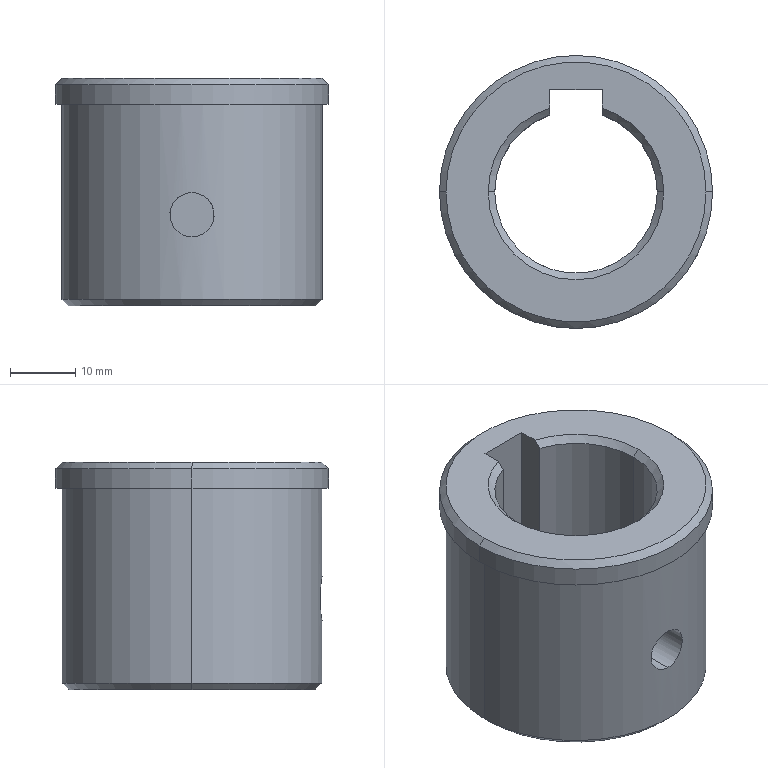Part | SolidWorks | features BaseBody 1 | 1 solid | 25 faces | box 42 x 42 x 35 mm | volume 25861 mm3 | cone 10 | cylinder 9 | plane 6 | commonest cylinder face diameters 25 x3 6.8 x2 40 x2 42 x2
STEP:
#1=CARTESIAN_POINT('',(0.,-12.5,-17.6));
#2=VERTEX_POINT('',#1);
#3=CARTESIAN_POINT('',(0.,-20.,-17.6));
#4=VERTEX_POINT('',#3);
#5=CARTESIAN_POINT('',(0.,-20.,-17.6));
#6=DIRECTION('',(0.,-1.,0.));
#7=VECTOR('',#6,1000.);
#8=LINE('',#5,#7);
#9=EDGE_CURVE('',#2,#4,#8,.T.);
#10=ORIENTED_EDGE('',*,*,#9,.F.);
#11=CARTESIAN_POINT('',(0.,-12.5,-24.4));
#12=VERTEX_POINT('',#11);
#13=CARTESIAN_POINT('',(0.,-12.5,-24.4));
#14=CARTESIAN_POINT('',(0.2239,-12.5,-24.4));
#15=CARTESIAN_POINT('',(0.446,-12.494,-24.378));
#16=CARTESIAN_POINT('',(0.8853,-12.471,-24.29));
#17=CARTESIAN_POINT('',(1.101,-12.453,-24.225));
#18=CARTESIAN_POINT('',(1.716,-12.388,-23.969));
#19=CARTESIAN_POINT('',(2.091,-12.328,-23.718));
#20=CARTESIAN_POINT('',(2.562,-12.236,-23.246));
#21=CARTESIAN_POINT('',(2.701,-12.205,-23.077));
#22=CARTESIAN_POINT('',(2.95,-12.148,-22.706));
#23=CARTESIAN_POINT('',(3.054,-12.122,-22.512));
#24=CARTESIAN_POINT('',(3.226,-12.077,-22.098));
#25=CARTESIAN_POINT('',(3.29,-12.059,-21.885));
#26=CARTESIAN_POINT('',(3.378,-12.035,-21.446));
#27=CARTESIAN_POINT('',(3.4,-12.029,-21.226));
#28=CARTESIAN_POINT('',(3.4,-12.029,-20.889));
#29=CARTESIAN_POINT('',(3.395,-12.03,-20.777));
#30=CARTESIAN_POINT('',(3.373,-12.036,-20.555));
#31=CARTESIAN_POINT('',(3.356,-12.041,-20.443));
#32=CARTESIAN_POINT('',(3.29,-12.059,-20.115));
#33=CARTESIAN_POINT('',(3.225,-12.077,-19.902));
#34=CARTESIAN_POINT('',(2.969,-12.144,-19.285));
#35=CARTESIAN_POINT('',(2.717,-12.205,-18.908));
#36=CARTESIAN_POINT('',(2.247,-12.297,-18.439));
#37=CARTESIAN_POINT('',(2.078,-12.328,-18.299));
#38=CARTESIAN_POINT('',(1.706,-12.384,-18.051));
#39=CARTESIAN_POINT('',(1.51,-12.41,-17.945));
#40=CARTESIAN_POINT('',(1.098,-12.453,-17.774));
#41=CARTESIAN_POINT('',(0.8878,-12.47,-17.71));
#42=CARTESIAN_POINT('',(0.4472,-12.494,-17.622));
#43=CARTESIAN_POINT('',(0.2246,-12.5,-17.6));
#44=CARTESIAN_POINT('',(0.,-12.5,-17.6));
#45=B_SPLINE_CURVE_WITH_KNOTS('',3,(#13,#14,#15,#16,#17,#18,#19,#20,#21,#22,#23,#24,#25,#26,#27,#28,#29,#30,#31,#32,#33,#34,#35,#36,#37,#38,#39,#40,#41,#42,#43,#44),.UNSPECIFIED.,.F.,.F.,(4,2,2,2,2,2,2,2,2,2,2,2,2,2,2,4),(0.,0.0625,0.125,0.25,0.3125,0.375,0.4375,0.5,0.5312,0.5625,0.625,0.75,0.8125,0.875,0.9375,1.),.UNSPECIFIED.);
#46=EDGE_CURVE('',#12,#2,#45,.T.);
#47=ORIENTED_EDGE('',*,*,#46,.F.);
#48=CARTESIAN_POINT('',(0.,-20.,-24.4));
#49=VERTEX_POINT('',#48);
#50=CARTESIAN_POINT('',(0.,-20.,-24.4));
#51=DIRECTION('',(0.,-1.,0.));
#52=VECTOR('',#51,1000.);
#53=LINE('',#50,#52);
#54=EDGE_CURVE('',#12,#49,#53,.T.);
#55=ORIENTED_EDGE('',*,*,#54,.T.);
#56=CARTESIAN_POINT('',(0.,-20.,-24.4));
#57=CARTESIAN_POINT('',(0.2109,-20.,-24.4));
#58=CARTESIAN_POINT('',(0.428,-19.996,-24.38));
#59=CARTESIAN_POINT('',(0.7563,-19.986,-24.317));
#60=CARTESIAN_POINT('',(0.8662,-19.981,-24.29));
#61=CARTESIAN_POINT('',(1.031,-19.973,-24.241));
#62=CARTESIAN_POINT('',(1.113,-19.969,-24.214));
#63=CARTESIAN_POINT('',(1.208,-19.963,-24.178));
#64=CARTESIAN_POINT('',(1.249,-19.961,-24.162));
#65=CARTESIAN_POINT('',(1.276,-19.959,-24.151));
#66=CARTESIAN_POINT('',(1.292,-19.958,-24.145));
#67=CARTESIAN_POINT('',(1.396,-19.951,-24.102));
#68=CARTESIAN_POINT('',(1.492,-19.945,-24.057));
#69=CARTESIAN_POINT('',(1.639,-19.933,-23.979));
#70=CARTESIAN_POINT('',(1.688,-19.929,-23.952));
#71=CARTESIAN_POINT('',(1.763,-19.922,-23.907));
#72=CARTESIAN_POINT('',(1.801,-19.919,-23.884));
#73=CARTESIAN_POINT('',(1.845,-19.915,-23.856));
#74=CARTESIAN_POINT('',(1.867,-19.913,-23.842));
#75=CARTESIAN_POINT('',(1.876,-19.912,-23.835));
#76=CARTESIAN_POINT('',(1.883,-19.911,-23.831));
#77=CARTESIAN_POINT('',(1.887,-19.911,-23.828));
#78=CARTESIAN_POINT('',(1.952,-19.905,-23.785));
#79=CARTESIAN_POINT('',(2.029,-19.897,-23.731));
#80=CARTESIAN_POINT('',(2.203,-19.878,-23.592));
#81=CARTESIAN_POINT('',(2.299,-19.868,-23.509));
#82=CARTESIAN_POINT('',(2.51,-19.842,-23.298));
#83=CARTESIAN_POINT('',(2.595,-19.831,-23.2));
#84=CARTESIAN_POINT('',(2.698,-19.817,-23.07));
#85=CARTESIAN_POINT('',(2.729,-19.813,-23.029));
#86=CARTESIAN_POINT('',(2.769,-19.807,-22.973));
#87=CARTESIAN_POINT('',(2.788,-19.805,-22.946));
#88=CARTESIAN_POINT('',(2.808,-19.802,-22.918));
#89=CARTESIAN_POINT('',(2.817,-19.801,-22.904));
#90=CARTESIAN_POINT('',(2.821,-19.8,-22.898));
#91=CARTESIAN_POINT('',(2.824,-19.8,-22.894));
#92=CARTESIAN_POINT('',(2.824,-19.8,-22.894));
#93=CARTESIAN_POINT('',(2.894,-19.79,-22.789));
#94=CARTESIAN_POINT('',(2.954,-19.781,-22.688));
#95=CARTESIAN_POINT('',(3.032,-19.769,-22.54));
#96=CARTESIAN_POINT('',(3.056,-19.765,-22.492));
#97=CARTESIAN_POINT('',(3.089,-19.76,-22.42));
#98=CARTESIAN_POINT('',(3.106,-19.757,-22.384));
#99=CARTESIAN_POINT('',(3.121,-19.755,-22.349));
#100=CARTESIAN_POINT('',(3.131,-19.753,-22.326));
#101=CARTESIAN_POINT('',(3.135,-19.753,-22.316));
#102=CARTESIAN_POINT('',(3.321,-19.723,-21.868));
#103=CARTESIAN_POINT('',(3.4,-19.709,-21.422));
#104=CARTESIAN_POINT('',(3.4,-19.709,-20.791));
#105=CARTESIAN_POINT('',(3.381,-19.712,-20.574));
#106=CARTESIAN_POINT('',(3.317,-19.723,-20.246));
#107=CARTESIAN_POINT('',(3.29,-19.728,-20.136));
#108=CARTESIAN_POINT('',(3.241,-19.736,-19.972));
#109=CARTESIAN_POINT('',(3.214,-19.74,-19.89));
#110=CARTESIAN_POINT('',(3.179,-19.746,-19.794));
#111=CARTESIAN_POINT('',(3.163,-19.748,-19.753));
#112=CARTESIAN_POINT('',(3.152,-19.75,-19.726));
#113=CARTESIAN_POINT('',(3.146,-19.751,-19.71));
#114=CARTESIAN_POINT('',(3.103,-19.758,-19.606));
#115=CARTESIAN_POINT('',(3.058,-19.765,-19.51));
#116=CARTESIAN_POINT('',(2.98,-19.777,-19.362));
#117=CARTESIAN_POINT('',(2.952,-19.781,-19.312));
#118=CARTESIAN_POINT('',(2.907,-19.788,-19.237));
#119=CARTESIAN_POINT('',(2.884,-19.791,-19.199));
#120=CARTESIAN_POINT('',(2.856,-19.795,-19.155));
#121=CARTESIAN_POINT('',(2.841,-19.797,-19.132));
#122=CARTESIAN_POINT('',(2.835,-19.798,-19.123));
#123=CARTESIAN_POINT('',(2.831,-19.799,-19.117));
#124=CARTESIAN_POINT('',(2.828,-19.799,-19.112));
#125=CARTESIAN_POINT('',(2.786,-19.805,-19.05));
#126=CARTESIAN_POINT('',(2.733,-19.813,-18.974));
#127=CARTESIAN_POINT('',(2.629,-19.827,-18.844));
#128=CARTESIAN_POINT('',(2.591,-19.832,-18.797));
#129=CARTESIAN_POINT('',(2.505,-19.843,-18.7));
#130=CARTESIAN_POINT('',(2.456,-19.849,-18.647));
#131=CARTESIAN_POINT('',(2.301,-19.867,-18.493));
#132=CARTESIAN_POINT('',(2.203,-19.878,-18.408));
#133=CARTESIAN_POINT('',(2.073,-19.892,-18.305));
#134=CARTESIAN_POINT('',(2.032,-19.896,-18.274));
#135=CARTESIAN_POINT('',(1.976,-19.902,-18.233));
#136=CARTESIAN_POINT('',(1.949,-19.905,-18.214));
#137=CARTESIAN_POINT('',(1.919,-19.908,-18.193));
#138=CARTESIAN_POINT('',(1.905,-19.909,-18.184));
#139=CARTESIAN_POINT('',(1.899,-19.91,-18.179));
#140=CARTESIAN_POINT('',(1.895,-19.91,-18.177));
#141=CARTESIAN_POINT('',(1.894,-19.91,-18.176));
#142=CARTESIAN_POINT('',(1.789,-19.92,-18.106));
#143=CARTESIAN_POINT('',(1.688,-19.929,-18.047));
#144=CARTESIAN_POINT('',(1.541,-19.941,-17.969));
#145=CARTESIAN_POINT('',(1.492,-19.944,-17.944));
#146=CARTESIAN_POINT('',(1.42,-19.95,-17.911));
#147=CARTESIAN_POINT('',(1.384,-19.952,-17.894));
#148=CARTESIAN_POINT('',(1.349,-19.954,-17.879));
#149=CARTESIAN_POINT('',(1.325,-19.956,-17.869));
#150=CARTESIAN_POINT('',(1.316,-19.957,-17.865));
#151=CARTESIAN_POINT('',(0.8685,-19.986,-17.679));
#152=CARTESIAN_POINT('',(0.4214,-20.,-17.6));
#153=CARTESIAN_POINT('',(0.,-20.,-17.6));
#154=B_SPLINE_CURVE_WITH_KNOTS('',3,(#56,#57,#58,#59,#60,#61,#62,#63,#64,#65,#66,#67,#68,#69,#70,#71,#72,#73,#74,#75,#76,#77,#78,#79,#80,#81,#82,#83,#84,#85,#86,#87,#88,#89,#90,#91,#92,#93,#94,#95,#96,#97,#98,#99,#100,#101,#102,#103,#104,#105,#106,#107,#108,#109,#110,#111,#112,#113,#114,#115,#116,#117,#118,#119,#120,#121,#122,#123,#124,#125,#126,#127,#128,#129,#130,#131,#132,#133,#134,#135,#136,#137,#138,#139,#140,#141,#142,#143,#144,#145,#146,#147,#148,#149,#150,#151,#152,#153),.UNSPECIFIED.,.F.,.F.,(4,2,2,1,1,2,2,2,2,1,1,1,2,2,2,2,2,2,1,1,1,2,2,2,2,1,2,2,2,2,2,1,1,2,2,2,2,1,1,1,2,2,2,2,2,2,2,1,1,1,2,2,2,2,1,2,2,4),(0.,0.0625,0.09375,0.1094,0.1172,0.1211,0.125,0.1563,0.1719,0.1797,0.1836,0.1855,0.1865,0.1875,0.2188,0.25,0.2813,0.2969,0.3047,0.3086,0.3105,0.3115,0.3125,0.3438,0.3594,0.3672,0.3711,0.375,0.5,0.5625,0.5938,0.6094,0.6172,0.6211,0.625,0.6563,0.6719,0.6797,0.6836,0.6855,0.6865,0.6875,0.7188,0.7344,0.75,0.7813,0.7969,0.8047,0.8086,0.8105,0.8115,0.8125,0.8438,0.8594,0.8672,0.8711,0.875,1.),.UNSPECIFIED.);
#155=EDGE_CURVE('',#49,#4,#154,.T.);
#156=ORIENTED_EDGE('',*,*,#155,.T.);
#157=EDGE_LOOP('',(#10,#47,#55,#156));
#158=FACE_OUTER_BOUND('',#157,.T.);
#159=CARTESIAN_POINT('',(0.,-20.,-21.));
#160=DIRECTION('',(0.,-1.,0.));
#161=DIRECTION('',(0.,0.,-1.));
#162=AXIS2_PLACEMENT_3D('',#159,#160,#161);
#163=CYLINDRICAL_SURFACE('',#162,3.4);
#164=ADVANCED_FACE('',(#158),#163,.F.);
#165=CARTESIAN_POINT('',(-19.,0.,-35.));
#166=VERTEX_POINT('',#165);
#167=CARTESIAN_POINT('',(-20.,0.,-34.));
#168=VERTEX_POINT('',#167);
#169=CARTESIAN_POINT('',(-20.,0.,-34.));
#170=DIRECTION('',(-0.7071,0.,0.7071));
#171=VECTOR('',#170,1000.);
#172=LINE('',#169,#171);
#173=EDGE_CURVE('',#166,#168,#172,.T.);
#174=ORIENTED_EDGE('',*,*,#173,.F.);
#175=CARTESIAN_POINT('',(19.,0.,-35.));
#176=VERTEX_POINT('',#175);
#177=CARTESIAN_POINT('',(0.,0.,-35.));
#178=DIRECTION('',(0.,0.,-1.));
#179=DIRECTION('',(1.,0.,0.));
#180=AXIS2_PLACEMENT_3D('',#177,#178,#179);
#181=CIRCLE('',#180,19.);
#182=EDGE_CURVE('',#176,#166,#181,.T.);
#183=ORIENTED_EDGE('',*,*,#182,.F.);
#184=CARTESIAN_POINT('',(20.,0.,-34.));
#185=VERTEX_POINT('',#184);
#186=CARTESIAN_POINT('',(20.,0.,-34.));
#187=DIRECTION('',(0.7071,0.,0.7071));
#188=VECTOR('',#187,1000.);
#189=LINE('',#186,#188);
#190=EDGE_CURVE('',#176,#185,#189,.T.);
#191=ORIENTED_EDGE('',*,*,#190,.T.);
#192=CARTESIAN_POINT('',(0.,0.,-34.));
#193=DIRECTION('',(0.,0.,1.));
#194=DIRECTION('',(1.,0.,0.));
#195=AXIS2_PLACEMENT_3D('',#192,#193,#194);
#196=CIRCLE('',#195,20.);
#197=EDGE_CURVE('',#168,#185,#196,.T.);
#198=ORIENTED_EDGE('',*,*,#197,.F.);
#199=EDGE_LOOP('',(#174,#183,#191,#198));
#200=FACE_OUTER_BOUND('',#199,.T.);
#201=CARTESIAN_POINT('',(0.,0.,-34.));
#202=DIRECTION('',(0.,0.,1.));
#203=DIRECTION('',(1.,0.,0.));
#204=AXIS2_PLACEMENT_3D('',#201,#202,#203);
#205=CONICAL_SURFACE('',#204,20.,0.7854);
#206=ADVANCED_FACE('',(#200),#205,.T.);
#207=CARTESIAN_POINT('',(12.5,0.,-34.));
#208=VERTEX_POINT('',#207);
#209=CARTESIAN_POINT('',(13.5,0.,-35.));
#210=VERTEX_POINT('',#209);
#211=CARTESIAN_POINT('',(13.5,0.,-35.));
#212=DIRECTION('',(0.7071,0.,-0.7071));
#213=VECTOR('',#212,1000.);
#214=LINE('',#211,#213);
#215=EDGE_CURVE('',#208,#210,#214,.T.);
#216=ORIENTED_EDGE('',*,*,#215,.F.);
#217=CARTESIAN_POINT('',(4.,11.843,-34.));
#218=VERTEX_POINT('',#217);
#219=CARTESIAN_POINT('',(0.,0.,-34.));
#220=DIRECTION('',(0.,0.,-1.));
#221=DIRECTION('',(1.,0.,0.));
#222=AXIS2_PLACEMENT_3D('',#219,#220,#221);
#223=CIRCLE('',#222,12.5);
#224=EDGE_CURVE('',#218,#208,#223,.T.);
#225=ORIENTED_EDGE('',*,*,#224,.F.);
#226=CARTESIAN_POINT('',(4.,12.894,-35.));
#227=VERTEX_POINT('',#226);
#228=CARTESIAN_POINT('',(4.,12.894,-35.));
#229=CARTESIAN_POINT('',(4.,12.544,-34.666));
#230=CARTESIAN_POINT('',(4.,12.194,-34.333));
#231=CARTESIAN_POINT('',(4.,11.843,-34.));
#232=B_SPLINE_CURVE_WITH_KNOTS('',3,(#228,#229,#230,#231),.UNSPECIFIED.,.F.,.F.,(4,4),(0.,0.001451),.UNSPECIFIED.);
#233=EDGE_CURVE('',#227,#218,#232,.T.);
#234=ORIENTED_EDGE('',*,*,#233,.F.);
#235=CARTESIAN_POINT('',(0.,0.,-35.));
#236=DIRECTION('',(0.,0.,1.));
#237=DIRECTION('',(1.,0.,0.));
#238=AXIS2_PLACEMENT_3D('',#235,#236,#237);
#239=CIRCLE('',#238,13.5);
#240=EDGE_CURVE('',#210,#227,#239,.T.);
#241=ORIENTED_EDGE('',*,*,#240,.F.);
#242=EDGE_LOOP('',(#216,#225,#234,#241));
#243=FACE_OUTER_BOUND('',#242,.T.);
#244=CARTESIAN_POINT('',(0.,0.,-35.));
#245=DIRECTION('',(0.,0.,-1.));
#246=DIRECTION('',(-1.,0.,0.));
#247=AXIS2_PLACEMENT_3D('',#244,#245,#246);
#248=CONICAL_SURFACE('',#247,13.5,0.7854);
#249=ADVANCED_FACE('',(#243),#248,.F.);
#250=CARTESIAN_POINT('',(-12.5,0.,-1.));
#251=VERTEX_POINT('',#250);
#252=CARTESIAN_POINT('',(-13.5,0.,0.));
#253=VERTEX_POINT('',#252);
#254=CARTESIAN_POINT('',(-12.5,0.,-1.));
#255=DIRECTION('',(-0.7071,0.,0.7071));
#256=VECTOR('',#255,1000.);
#257=LINE('',#254,#256);
#258=EDGE_CURVE('',#251,#253,#257,.T.);
#259=ORIENTED_EDGE('',*,*,#258,.F.);
#260=CARTESIAN_POINT('',(-4.,11.843,-1.));
#261=VERTEX_POINT('',#260);
#262=CARTESIAN_POINT('',(0.,0.,-1.));
#263=DIRECTION('',(0.,0.,1.));
#264=DIRECTION('',(1.,0.,0.));
#265=AXIS2_PLACEMENT_3D('',#262,#263,#264);
#266=CIRCLE('',#265,12.5);
#267=EDGE_CURVE('',#261,#251,#266,.T.);
#268=ORIENTED_EDGE('',*,*,#267,.F.);
#269=CARTESIAN_POINT('',(-4.,12.894,0.));
#270=VERTEX_POINT('',#269);
#271=CARTESIAN_POINT('',(-4.,12.894,0.));
#272=CARTESIAN_POINT('',(-4.,12.544,-0.334));
#273=CARTESIAN_POINT('',(-4.,12.194,-0.6674));
#274=CARTESIAN_POINT('',(-4.,11.843,-1.));
#275=B_SPLINE_CURVE_WITH_KNOTS('',3,(#271,#272,#273,#274),.UNSPECIFIED.,.F.,.F.,(4,4),(0.,0.001451),.UNSPECIFIED.);
#276=EDGE_CURVE('',#270,#261,#275,.T.);
#277=ORIENTED_EDGE('',*,*,#276,.F.);
#278=CARTESIAN_POINT('',(0.,0.,0.));
#279=DIRECTION('',(0.,0.,-1.));
#280=DIRECTION('',(1.,0.,0.));
#281=AXIS2_PLACEMENT_3D('',#278,#279,#280);
#282=CIRCLE('',#281,13.5);
#283=EDGE_CURVE('',#253,#270,#282,.T.);
#284=ORIENTED_EDGE('',*,*,#283,.F.);
#285=EDGE_LOOP('',(#259,#268,#277,#284));
#286=FACE_OUTER_BOUND('',#285,.T.);
#287=CARTESIAN_POINT('',(0.,0.,-1.));
#288=DIRECTION('',(0.,0.,1.));
#289=DIRECTION('',(1.,0.,0.));
#290=AXIS2_PLACEMENT_3D('',#287,#288,#289);
#291=CONICAL_SURFACE('',#290,12.5,0.7854);
#292=ADVANCED_FACE('',(#286),#291,.F.);
#293=CARTESIAN_POINT('',(20.,0.,0.));
#294=VERTEX_POINT('',#293);
#295=CARTESIAN_POINT('',(21.,0.,-1.));
#296=VERTEX_POINT('',#295);
#297=CARTESIAN_POINT('',(20.,0.,0.));
#298=DIRECTION('',(0.7071,0.,-0.7071));
#299=VECTOR('',#298,1000.);
#300=LINE('',#297,#299);
#301=EDGE_CURVE('',#294,#296,#300,.T.);
#302=ORIENTED_EDGE('',*,*,#301,.F.);
#303=CARTESIAN_POINT('',(-20.,0.,0.));
#304=VERTEX_POINT('',#303);
#305=CARTESIAN_POINT('',(0.,0.,0.));
#306=DIRECTION('',(0.,0.,1.));
#307=DIRECTION('',(1.,0.,0.));
#308=AXIS2_PLACEMENT_3D('',#305,#306,#307);
#309=CIRCLE('',#308,20.);
#310=EDGE_CURVE('',#304,#294,#309,.T.);
#311=ORIENTED_EDGE('',*,*,#310,.F.);
#312=CARTESIAN_POINT('',(-21.,0.,-1.));
#313=VERTEX_POINT('',#312);
#314=CARTESIAN_POINT('',(-20.,0.,0.));
#315=DIRECTION('',(-0.7071,0.,-0.7071));
#316=VECTOR('',#315,1000.);
#317=LINE('',#314,#316);
#318=EDGE_CURVE('',#304,#313,#317,.T.);
#319=ORIENTED_EDGE('',*,*,#318,.T.);
#320=CARTESIAN_POINT('',(0.,0.,-1.));
#321=DIRECTION('',(0.,0.,-1.));
#322=DIRECTION('',(1.,0.,0.));
#323=AXIS2_PLACEMENT_3D('',#320,#321,#322);
#324=CIRCLE('',#323,21.);
#325=EDGE_CURVE('',#296,#313,#324,.T.);
#326=ORIENTED_EDGE('',*,*,#325,.F.);
#327=EDGE_LOOP('',(#302,#311,#319,#326));
#328=FACE_OUTER_BOUND('',#327,.T.);
#329=CARTESIAN_POINT('',(0.,0.,0.));
#330=DIRECTION('',(0.,0.,-1.));
#331=DIRECTION('',(-1.,0.,0.));
#332=AXIS2_PLACEMENT_3D('',#329,#330,#331);
#333=CONICAL_SURFACE('',#332,20.,0.7854);
#334=ADVANCED_FACE('',(#328),#333,.T.);
#335=CARTESIAN_POINT('',(-4.,15.8,-35.));
#336=VERTEX_POINT('',#335);
#337=CARTESIAN_POINT('',(4.,15.8,-35.));
#338=VERTEX_POINT('',#337);
#339=CARTESIAN_POINT('',(4.,15.8,-35.));
#340=DIRECTION('',(1.,0.,0.));
#341=VECTOR('',#340,1000.);
#342=LINE('',#339,#341);
#343=EDGE_CURVE('',#336,#338,#342,.T.);
#344=ORIENTED_EDGE('',*,*,#343,.T.);
#345=CARTESIAN_POINT('',(4.,15.8,0.));
#346=VERTEX_POINT('',#345);
#347=CARTESIAN_POINT('',(4.,15.8,0.));
#348=DIRECTION('',(0.,0.,-1.));
#349=VECTOR('',#348,1000.);
#350=LINE('',#347,#349);
#351=EDGE_CURVE('',#346,#338,#350,.T.);
#352=ORIENTED_EDGE('',*,*,#351,.F.);
#353=CARTESIAN_POINT('',(-4.,15.8,0.));
#354=VERTEX_POINT('',#353);
#355=CARTESIAN_POINT('',(4.,15.8,0.));
#356=DIRECTION('',(1.,0.,0.));
#357=VECTOR('',#356,1000.);
#358=LINE('',#355,#357);
#359=EDGE_CURVE('',#354,#346,#358,.T.);
#360=ORIENTED_EDGE('',*,*,#359,.F.);
#361=CARTESIAN_POINT('',(-4.,15.8,0.));
#362=DIRECTION('',(0.,0.,-1.));
#363=VECTOR('',#362,1000.);
#364=LINE('',#361,#363);
#365=EDGE_CURVE('',#354,#336,#364,.T.);
#366=ORIENTED_EDGE('',*,*,#365,.T.);
#367=EDGE_LOOP('',(#344,#352,#360,#366));
#368=FACE_OUTER_BOUND('',#367,.T.);
#369=CARTESIAN_POINT('',(4.,15.8,0.));
#370=DIRECTION('',(0.,1.,0.));
#371=DIRECTION('',(1.,0.,0.));
#372=AXIS2_PLACEMENT_3D('',#369,#370,#371);
#373=PLANE('',#372);
#374=ADVANCED_FACE('',(#368),#373,.F.);
#375=CARTESIAN_POINT('',(4.,11.843,-1.));
#376=VERTEX_POINT('',#375);
#377=CARTESIAN_POINT('',(4.,11.843,-35.));
#378=DIRECTION('',(0.,0.,-1.));
#379=VECTOR('',#378,1000.);
#380=LINE('',#377,#379);
#381=EDGE_CURVE('',#376,#218,#380,.T.);
#382=ORIENTED_EDGE('',*,*,#381,.F.);
#383=CARTESIAN_POINT('',(4.,12.894,0.));
#384=VERTEX_POINT('',#383);
#385=CARTESIAN_POINT('',(4.,11.843,-1.));
#386=CARTESIAN_POINT('',(4.,12.194,-0.6674));
#387=CARTESIAN_POINT('',(4.,12.544,-0.334));
#388=CARTESIAN_POINT('',(4.,12.894,0.));
#389=B_SPLINE_CURVE_WITH_KNOTS('',3,(#385,#386,#387,#388),.UNSPECIFIED.,.F.,.F.,(4,4),(0.,0.001451),.UNSPECIFIED.);
#390=EDGE_CURVE('',#376,#384,#389,.T.);
#391=ORIENTED_EDGE('',*,*,#390,.T.);
#392=CARTESIAN_POINT('',(4.,15.8,0.));
#393=DIRECTION('',(0.,-1.,0.));
#394=VECTOR('',#393,1000.);
#395=LINE('',#392,#394);
#396=EDGE_CURVE('',#346,#384,#395,.T.);
#397=ORIENTED_EDGE('',*,*,#396,.F.);
#398=ORIENTED_EDGE('',*,*,#351,.T.);
#399=CARTESIAN_POINT('',(4.,15.8,-35.));
#400=DIRECTION('',(0.,-1.,0.));
#401=VECTOR('',#400,1000.);
#402=LINE('',#399,#401);
#403=EDGE_CURVE('',#338,#227,#402,.T.);
#404=ORIENTED_EDGE('',*,*,#403,.T.);
#405=ORIENTED_EDGE('',*,*,#233,.T.);
#406=EDGE_LOOP('',(#382,#391,#397,#398,#404,#405));
#407=FACE_OUTER_BOUND('',#406,.T.);
#408=CARTESIAN_POINT('',(4.,15.8,0.));
#409=DIRECTION('',(1.,0.,0.));
#410=DIRECTION('',(0.,1.,0.));
#411=AXIS2_PLACEMENT_3D('',#408,#409,#410);
#412=PLANE('',#411);
#413=ADVANCED_FACE('',(#407),#412,.F.);
#414=CARTESIAN_POINT('',(-4.,15.8,0.));
#415=DIRECTION('',(0.,1.,0.));
#416=VECTOR('',#415,1000.);
#417=LINE('',#414,#416);
#418=EDGE_CURVE('',#270,#354,#417,.T.);
#419=ORIENTED_EDGE('',*,*,#418,.F.);
#420=ORIENTED_EDGE('',*,*,#276,.T.);
#421=CARTESIAN_POINT('',(-4.,11.843,-34.));
#422=VERTEX_POINT('',#421);
#423=CARTESIAN_POINT('',(-4.,11.843,-35.));
#424=DIRECTION('',(0.,0.,1.));
#425=VECTOR('',#424,1000.);
#426=LINE('',#423,#425);
#427=EDGE_CURVE('',#422,#261,#426,.T.);
#428=ORIENTED_EDGE('',*,*,#427,.F.);
#429=CARTESIAN_POINT('',(-4.,12.894,-35.));
#430=VERTEX_POINT('',#429);
#431=CARTESIAN_POINT('',(-4.,11.843,-34.));
#432=CARTESIAN_POINT('',(-4.,12.194,-34.333));
#433=CARTESIAN_POINT('',(-4.,12.544,-34.666));
#434=CARTESIAN_POINT('',(-4.,12.894,-35.));
#435=B_SPLINE_CURVE_WITH_KNOTS('',3,(#431,#432,#433,#434),.UNSPECIFIED.,.F.,.F.,(4,4),(0.,0.001451),.UNSPECIFIED.);
#436=EDGE_CURVE('',#422,#430,#435,.T.);
#437=ORIENTED_EDGE('',*,*,#436,.T.);
#438=CARTESIAN_POINT('',(-4.,15.8,-35.));
#439=DIRECTION('',(0.,1.,0.));
#440=VECTOR('',#439,1000.);
#441=LINE('',#438,#440);
#442=EDGE_CURVE('',#430,#336,#441,.T.);
#443=ORIENTED_EDGE('',*,*,#442,.T.);
#444=ORIENTED_EDGE('',*,*,#365,.F.);
#445=EDGE_LOOP('',(#419,#420,#428,#437,#443,#444));
#446=FACE_OUTER_BOUND('',#445,.T.);
#447=CARTESIAN_POINT('',(-4.,15.8,0.));
#448=DIRECTION('',(-1.,0.,0.));
#449=DIRECTION('',(0.,0.,1.));
#450=AXIS2_PLACEMENT_3D('',#447,#448,#449);
#451=PLANE('',#450);
#452=ADVANCED_FACE('',(#446),#451,.F.);
#453=CARTESIAN_POINT('',(20.,0.,-4.));
#454=VERTEX_POINT('',#453);
#455=CARTESIAN_POINT('',(-20.,0.,-4.));
#456=VERTEX_POINT('',#455);
#457=CARTESIAN_POINT('',(0.,0.,-4.));
#458=DIRECTION('',(0.,0.,-1.));
#459=DIRECTION('',(1.,0.,0.));
#460=AXIS2_PLACEMENT_3D('',#457,#458,#459);
#461=CIRCLE('',#460,20.);
#462=EDGE_CURVE('',#454,#456,#461,.T.);
#463=ORIENTED_EDGE('',*,*,#462,.F.);
#464=CARTESIAN_POINT('',(0.,0.,-4.));
#465=DIRECTION('',(0.,0.,-1.));
#466=DIRECTION('',(1.,0.,0.));
#467=AXIS2_PLACEMENT_3D('',#464,#465,#466);
#468=CIRCLE('',#467,20.);
#469=EDGE_CURVE('',#456,#454,#468,.T.);
#470=ORIENTED_EDGE('',*,*,#469,.F.);
#471=EDGE_LOOP('',(#463,#470));
#472=FACE_BOUND('',#471,.T.);
#473=CARTESIAN_POINT('',(21.,0.,-4.));
#474=VERTEX_POINT('',#473);
#475=CARTESIAN_POINT('',(-21.,0.,-4.));
#476=VERTEX_POINT('',#475);
#477=CARTESIAN_POINT('',(0.,0.,-4.));
#478=DIRECTION('',(0.,0.,1.));
#479=DIRECTION('',(1.,0.,0.));
#480=AXIS2_PLACEMENT_3D('',#477,#478,#479);
#481=CIRCLE('',#480,21.);
#482=EDGE_CURVE('',#474,#476,#481,.T.);
#483=ORIENTED_EDGE('',*,*,#482,.F.);
#484=CARTESIAN_POINT('',(0.,0.,-4.));
#485=DIRECTION('',(0.,0.,1.));
#486=DIRECTION('',(1.,0.,0.));
#487=AXIS2_PLACEMENT_3D('',#484,#485,#486);
#488=CIRCLE('',#487,21.);
#489=EDGE_CURVE('',#476,#474,#488,.T.);
#490=ORIENTED_EDGE('',*,*,#489,.F.);
#491=EDGE_LOOP('',(#483,#490));
#492=FACE_OUTER_BOUND('',#491,.T.);
#493=CARTESIAN_POINT('',(0.,0.,-4.));
#494=DIRECTION('',(0.,0.,1.));
#495=DIRECTION('',(1.,0.,0.));
#496=AXIS2_PLACEMENT_3D('',#493,#494,#495);
#497=PLANE('',#496);
#498=ADVANCED_FACE('',(#472,#492),#497,.F.);
#499=CARTESIAN_POINT('',(-21.,0.,-4.));
#500=DIRECTION('',(0.,0.,1.));
#501=VECTOR('',#500,1000.);
#502=LINE('',#499,#501);
#503=EDGE_CURVE('',#476,#313,#502,.T.);
#504=ORIENTED_EDGE('',*,*,#503,.F.);
#505=ORIENTED_EDGE('',*,*,#489,.T.);
#506=CARTESIAN_POINT('',(21.,0.,-4.));
#507=DIRECTION('',(0.,0.,1.));
#508=VECTOR('',#507,1000.);
#509=LINE('',#506,#508);
#510=EDGE_CURVE('',#474,#296,#509,.T.);
#511=ORIENTED_EDGE('',*,*,#510,.T.);
#512=ORIENTED_EDGE('',*,*,#325,.T.);
#513=EDGE_LOOP('',(#504,#505,#511,#512));
#514=FACE_OUTER_BOUND('',#513,.T.);
#515=CARTESIAN_POINT('',(0.,0.,-4.));
#516=DIRECTION('',(0.,0.,1.));
#517=DIRECTION('',(1.,0.,0.));
#518=AXIS2_PLACEMENT_3D('',#515,#516,#517);
#519=CYLINDRICAL_SURFACE('',#518,21.);
#520=ADVANCED_FACE('',(#514),#519,.T.);
#521=CARTESIAN_POINT('',(-12.5,0.,-34.));
#522=VERTEX_POINT('',#521);
#523=CARTESIAN_POINT('',(-12.5,0.,-35.));
#524=DIRECTION('',(0.,0.,1.));
#525=VECTOR('',#524,1000.);
#526=LINE('',#523,#525);
#527=EDGE_CURVE('',#522,#251,#526,.T.);
#528=ORIENTED_EDGE('',*,*,#527,.F.);
#529=CARTESIAN_POINT('',(0.,0.,-34.));
#530=DIRECTION('',(0.,0.,-1.));
#531=DIRECTION('',(1.,0.,0.));
#532=AXIS2_PLACEMENT_3D('',#529,#530,#531);
#533=CIRCLE('',#532,12.5);
#534=EDGE_CURVE('',#522,#422,#533,.T.);
#535=ORIENTED_EDGE('',*,*,#534,.T.);
#536=ORIENTED_EDGE('',*,*,#427,.T.);
#537=ORIENTED_EDGE('',*,*,#267,.T.);
#538=EDGE_LOOP('',(#528,#535,#536,#537));
#539=FACE_OUTER_BOUND('',#538,.T.);
#540=CARTESIAN_POINT('',(0.,0.,-35.));
#541=DIRECTION('',(0.,0.,1.));
#542=DIRECTION('',(1.,0.,0.));
#543=AXIS2_PLACEMENT_3D('',#540,#541,#542);
#544=CYLINDRICAL_SURFACE('',#543,12.5);
#545=ADVANCED_FACE('',(#539),#544,.F.);
#546=ORIENTED_EDGE('',*,*,#396,.T.);
#547=CARTESIAN_POINT('',(13.5,0.,0.));
#548=VERTEX_POINT('',#547);
#549=CARTESIAN_POINT('',(0.,0.,0.));
#550=DIRECTION('',(0.,0.,-1.));
#551=DIRECTION('',(1.,0.,0.));
#552=AXIS2_PLACEMENT_3D('',#549,#550,#551);
#553=CIRCLE('',#552,13.5);
#554=EDGE_CURVE('',#384,#548,#553,.T.);
#555=ORIENTED_EDGE('',*,*,#554,.T.);
#556=CARTESIAN_POINT('',(0.,0.,0.));
#557=DIRECTION('',(0.,0.,-1.));
#558=DIRECTION('',(1.,0.,0.));
#559=AXIS2_PLACEMENT_3D('',#556,#557,#558);
#560=CIRCLE('',#559,13.5);
#561=EDGE_CURVE('',#548,#253,#560,.T.);
#562=ORIENTED_EDGE('',*,*,#561,.T.);
#563=ORIENTED_EDGE('',*,*,#283,.T.);
#564=ORIENTED_EDGE('',*,*,#418,.T.);
#565=ORIENTED_EDGE('',*,*,#359,.T.);
#566=EDGE_LOOP('',(#546,#555,#562,#563,#564,#565));
#567=FACE_BOUND('',#566,.T.);
#568=ORIENTED_EDGE('',*,*,#310,.T.);
#569=CARTESIAN_POINT('',(0.,0.,0.));
#570=DIRECTION('',(0.,0.,1.));
#571=DIRECTION('',(1.,0.,0.));
#572=AXIS2_PLACEMENT_3D('',#569,#570,#571);
#573=CIRCLE('',#572,20.);
#574=EDGE_CURVE('',#294,#304,#573,.T.);
#575=ORIENTED_EDGE('',*,*,#574,.T.);
#576=EDGE_LOOP('',(#568,#575));
#577=FACE_OUTER_BOUND('',#576,.T.);
#578=CARTESIAN_POINT('',(0.,0.,0.));
#579=DIRECTION('',(0.,0.,1.));
#580=DIRECTION('',(1.,0.,0.));
#581=AXIS2_PLACEMENT_3D('',#578,#579,#580);
#582=PLANE('',#581);
#583=ADVANCED_FACE('',(#567,#577),#582,.T.);
#584=ORIENTED_EDGE('',*,*,#442,.F.);
#585=CARTESIAN_POINT('',(-13.5,0.,-35.));
#586=VERTEX_POINT('',#585);
#587=CARTESIAN_POINT('',(0.,0.,-35.));
#588=DIRECTION('',(0.,0.,1.));
#589=DIRECTION('',(1.,0.,0.));
#590=AXIS2_PLACEMENT_3D('',#587,#588,#589);
#591=CIRCLE('',#590,13.5);
#592=EDGE_CURVE('',#430,#586,#591,.T.);
#593=ORIENTED_EDGE('',*,*,#592,.T.);
#594=CARTESIAN_POINT('',(0.,0.,-35.));
#595=DIRECTION('',(0.,0.,1.));
#596=DIRECTION('',(1.,0.,0.));
#597=AXIS2_PLACEMENT_3D('',#594,#595,#596);
#598=CIRCLE('',#597,13.5);
#599=EDGE_CURVE('',#586,#210,#598,.T.);
#600=ORIENTED_EDGE('',*,*,#599,.T.);
#601=ORIENTED_EDGE('',*,*,#240,.T.);
#602=ORIENTED_EDGE('',*,*,#403,.F.);
#603=ORIENTED_EDGE('',*,*,#343,.F.);
#604=EDGE_LOOP('',(#584,#593,#600,#601,#602,#603));
#605=FACE_BOUND('',#604,.T.);
#606=ORIENTED_EDGE('',*,*,#182,.T.);
#607=CARTESIAN_POINT('',(0.,0.,-35.));
#608=DIRECTION('',(0.,0.,-1.));
#609=DIRECTION('',(1.,0.,0.));
#610=AXIS2_PLACEMENT_3D('',#607,#608,#609);
#611=CIRCLE('',#610,19.);
#612=EDGE_CURVE('',#166,#176,#611,.T.);
#613=ORIENTED_EDGE('',*,*,#612,.T.);
#614=EDGE_LOOP('',(#606,#613));
#615=FACE_OUTER_BOUND('',#614,.T.);
#616=CARTESIAN_POINT('',(0.,0.,-35.));
#617=DIRECTION('',(0.,0.,1.));
#618=DIRECTION('',(1.,0.,0.));
#619=AXIS2_PLACEMENT_3D('',#616,#617,#618);
#620=PLANE('',#619);
#621=ADVANCED_FACE('',(#605,#615),#620,.F.);
#622=ORIENTED_EDGE('',*,*,#155,.F.);
#623=CARTESIAN_POINT('',(0.,-20.,-17.6));
#624=CARTESIAN_POINT('',(-0.2106,-20.,-17.6));
#625=CARTESIAN_POINT('',(-0.4273,-19.996,-17.62));
#626=CARTESIAN_POINT('',(-0.7551,-19.986,-17.683));
#627=CARTESIAN_POINT('',(-0.8649,-19.981,-17.71));
#628=CARTESIAN_POINT('',(-1.029,-19.974,-17.759));
#629=CARTESIAN_POINT('',(-1.111,-19.969,-17.786));
#630=CARTESIAN_POINT('',(-1.206,-19.964,-17.821));
#631=CARTESIAN_POINT('',(-1.247,-19.961,-17.837));
#632=CARTESIAN_POINT('',(-1.274,-19.959,-17.848));
#633=CARTESIAN_POINT('',(-1.29,-19.958,-17.854));
#634=CARTESIAN_POINT('',(-1.394,-19.952,-17.897));
#635=CARTESIAN_POINT('',(-1.491,-19.945,-17.942));
#636=CARTESIAN_POINT('',(-1.638,-19.933,-18.02));
#637=CARTESIAN_POINT('',(-1.688,-19.929,-18.048));
#638=CARTESIAN_POINT('',(-1.763,-19.922,-18.093));
#639=CARTESIAN_POINT('',(-1.801,-19.919,-18.116));
#640=CARTESIAN_POINT('',(-1.845,-19.915,-18.144));
#641=CARTESIAN_POINT('',(-1.867,-19.913,-18.159));
#642=CARTESIAN_POINT('',(-1.877,-19.912,-18.165));
#643=CARTESIAN_POINT('',(-1.883,-19.911,-18.169));
#644=CARTESIAN_POINT('',(-1.888,-19.911,-18.172));
#645=CARTESIAN_POINT('',(-1.953,-19.905,-18.216));
#646=CARTESIAN_POINT('',(-2.029,-19.897,-18.27));
#647=CARTESIAN_POINT('',(-2.159,-19.883,-18.373));
#648=CARTESIAN_POINT('',(-2.205,-19.878,-18.411));
#649=CARTESIAN_POINT('',(-2.301,-19.867,-18.496));
#650=CARTESIAN_POINT('',(-2.35,-19.862,-18.541));
#651=CARTESIAN_POINT('',(-2.509,-19.842,-18.7));
#652=CARTESIAN_POINT('',(-2.594,-19.831,-18.799));
#653=CARTESIAN_POINT('',(-2.698,-19.817,-18.93));
#654=CARTESIAN_POINT('',(-2.729,-19.813,-18.971));
#655=CARTESIAN_POINT('',(-2.769,-19.807,-19.027));
#656=CARTESIAN_POINT('',(-2.788,-19.805,-19.054));
#657=CARTESIAN_POINT('',(-2.808,-19.802,-19.082));
#658=CARTESIAN_POINT('',(-2.817,-19.801,-19.096));
#659=CARTESIAN_POINT('',(-2.821,-19.8,-19.102));
#660=CARTESIAN_POINT('',(-2.824,-19.8,-19.106));
#661=CARTESIAN_POINT('',(-2.824,-19.8,-19.107));
#662=CARTESIAN_POINT('',(-2.894,-19.79,-19.211));
#663=CARTESIAN_POINT('',(-2.953,-19.781,-19.311));
#664=CARTESIAN_POINT('',(-3.031,-19.769,-19.458));
#665=CARTESIAN_POINT('',(-3.055,-19.765,-19.507));
#666=CARTESIAN_POINT('',(-3.089,-19.76,-19.578));
#667=CARTESIAN_POINT('',(-3.105,-19.758,-19.614));
#668=CARTESIAN_POINT('',(-3.122,-19.755,-19.655));
#669=CARTESIAN_POINT('',(-3.13,-19.754,-19.672));
#670=CARTESIAN_POINT('',(-3.135,-19.753,-19.683));
#671=CARTESIAN_POINT('',(-3.137,-19.752,-19.688));
#672=CARTESIAN_POINT('',(-3.32,-19.723,-20.13));
#673=CARTESIAN_POINT('',(-3.4,-19.709,-20.577));
#674=CARTESIAN_POINT('',(-3.4,-19.709,-21.208));
#675=CARTESIAN_POINT('',(-3.381,-19.712,-21.425));
#676=CARTESIAN_POINT('',(-3.317,-19.723,-21.753));
#677=CARTESIAN_POINT('',(-3.291,-19.728,-21.863));
#678=CARTESIAN_POINT('',(-3.241,-19.736,-22.028));
#679=CARTESIAN_POINT('',(-3.215,-19.74,-22.11));
#680=CARTESIAN_POINT('',(-3.179,-19.746,-22.206));
#681=CARTESIAN_POINT('',(-3.163,-19.748,-22.247));
#682=CARTESIAN_POINT('',(-3.152,-19.75,-22.274));
#683=CARTESIAN_POINT('',(-3.146,-19.751,-22.29));
#684=CARTESIAN_POINT('',(-3.103,-19.758,-22.393));
#685=CARTESIAN_POINT('',(-3.059,-19.765,-22.489));
#686=CARTESIAN_POINT('',(-2.981,-19.777,-22.636));
#687=CARTESIAN_POINT('',(-2.953,-19.781,-22.686));
#688=CARTESIAN_POINT('',(-2.909,-19.787,-22.761));
#689=CARTESIAN_POINT('',(-2.886,-19.791,-22.798));
#690=CARTESIAN_POINT('',(-2.858,-19.795,-22.842));
#691=CARTESIAN_POINT('',(-2.843,-19.797,-22.865));
#692=CARTESIAN_POINT('',(-2.837,-19.798,-22.874));
#693=CARTESIAN_POINT('',(-2.833,-19.798,-22.88));
#694=CARTESIAN_POINT('',(-2.83,-19.799,-22.885));
#695=CARTESIAN_POINT('',(-2.788,-19.805,-22.948));
#696=CARTESIAN_POINT('',(-2.735,-19.812,-23.023));
#697=CARTESIAN_POINT('',(-2.631,-19.826,-23.154));
#698=CARTESIAN_POINT('',(-2.592,-19.831,-23.201));
#699=CARTESIAN_POINT('',(-2.506,-19.842,-23.299));
#700=CARTESIAN_POINT('',(-2.457,-19.849,-23.351));
#701=CARTESIAN_POINT('',(-2.302,-19.867,-23.506));
#702=CARTESIAN_POINT('',(-2.205,-19.878,-23.59));
#703=CARTESIAN_POINT('',(-2.075,-19.892,-23.694));
#704=CARTESIAN_POINT('',(-2.034,-19.896,-23.725));
#705=CARTESIAN_POINT('',(-1.977,-19.902,-23.766));
#706=CARTESIAN_POINT('',(-1.95,-19.905,-23.785));
#707=CARTESIAN_POINT('',(-1.921,-19.908,-23.806));
#708=CARTESIAN_POINT('',(-1.906,-19.909,-23.815));
#709=CARTESIAN_POINT('',(-1.9,-19.909,-23.819));
#710=CARTESIAN_POINT('',(-1.897,-19.91,-23.822));
#711=CARTESIAN_POINT('',(-1.896,-19.91,-23.822));
#712=CARTESIAN_POINT('',(-1.791,-19.92,-23.892));
#713=CARTESIAN_POINT('',(-1.691,-19.929,-23.952));
#714=CARTESIAN_POINT('',(-1.544,-19.94,-24.03));
#715=CARTESIAN_POINT('',(-1.495,-19.944,-24.054));
#716=CARTESIAN_POINT('',(-1.423,-19.949,-24.088));
#717=CARTESIAN_POINT('',(-1.388,-19.952,-24.104));
#718=CARTESIAN_POINT('',(-1.352,-19.954,-24.119));
#719=CARTESIAN_POINT('',(-1.329,-19.956,-24.129));
#720=CARTESIAN_POINT('',(-1.319,-19.956,-24.134));
#721=CARTESIAN_POINT('',(-0.8711,-19.986,-24.32));
#722=CARTESIAN_POINT('',(-0.4226,-20.,-24.4));
#723=CARTESIAN_POINT('',(0.,-20.,-24.4));
#724=B_SPLINE_CURVE_WITH_KNOTS('',3,(#623,#624,#625,#626,#627,#628,#629,#630,#631,#632,#633,#634,#635,#636,#637,#638,#639,#640,#641,#642,#643,#644,#645,#646,#647,#648,#649,#650,#651,#652,#653,#654,#655,#656,#657,#658,#659,#660,#661,#662,#663,#664,#665,#666,#667,#668,#669,#670,#671,#672,#673,#674,#675,#676,#677,#678,#679,#680,#681,#682,#683,#684,#685,#686,#687,#688,#689,#690,#691,#692,#693,#694,#695,#696,#697,#698,#699,#700,#701,#702,#703,#704,#705,#706,#707,#708,#709,#710,#711,#712,#713,#714,#715,#716,#717,#718,#719,#720,#721,#722,#723),.UNSPECIFIED.,.F.,.F.,(4,2,2,1,1,2,2,2,2,1,1,1,2,2,2,2,2,2,2,1,1,1,2,2,2,2,1,1,2,2,2,2,2,1,1,2,2,2,2,1,1,1,2,2,2,2,2,2,2,1,1,1,2,2,2,2,1,2,2,4),(0.,0.0625,0.09375,0.1094,0.1172,0.1211,0.125,0.1563,0.1719,0.1797,0.1836,0.1855,0.1865,0.1875,0.2188,0.2344,0.25,0.2813,0.2969,0.3047,0.3086,0.3105,0.3115,0.3125,0.3438,0.3594,0.3672,0.3711,0.373,0.375,0.5,0.5625,0.5937,0.6094,0.6172,0.6211,0.625,0.6562,0.6719,0.6797,0.6836,0.6855,0.6865,0.6875,0.7187,0.7344,0.75,0.7812,0.7969,0.8047,0.8086,0.8105,0.8115,0.8125,0.8437,0.8594,0.8672,0.8711,0.875,1.),.UNSPECIFIED.);
#725=EDGE_CURVE('',#4,#49,#724,.T.);
#726=ORIENTED_EDGE('',*,*,#725,.F.);
#727=EDGE_LOOP('',(#622,#726));
#728=FACE_BOUND('',#727,.T.);
#729=CARTESIAN_POINT('',(-20.,0.,-35.));
#730=DIRECTION('',(0.,0.,1.));
#731=VECTOR('',#730,1000.);
#732=LINE('',#729,#731);
#733=EDGE_CURVE('',#168,#456,#732,.T.);
#734=ORIENTED_EDGE('',*,*,#733,.F.);
#735=ORIENTED_EDGE('',*,*,#197,.T.);
#736=CARTESIAN_POINT('',(20.,0.,-35.));
#737=DIRECTION('',(0.,0.,1.));
#738=VECTOR('',#737,1000.);
#739=LINE('',#736,#738);
#740=EDGE_CURVE('',#185,#454,#739,.T.);
#741=ORIENTED_EDGE('',*,*,#740,.T.);
#742=ORIENTED_EDGE('',*,*,#462,.T.);
#743=EDGE_LOOP('',(#734,#735,#741,#742));
#744=FACE_OUTER_BOUND('',#743,.T.);
#745=CARTESIAN_POINT('',(0.,0.,-35.));
#746=DIRECTION('',(0.,0.,1.));
#747=DIRECTION('',(1.,0.,0.));
#748=AXIS2_PLACEMENT_3D('',#745,#746,#747);
#749=CYLINDRICAL_SURFACE('',#748,20.);
#750=ADVANCED_FACE('',(#728,#744),#749,.T.);
#751=CARTESIAN_POINT('',(0.,0.,-34.));
#752=DIRECTION('',(0.,0.,1.));
#753=DIRECTION('',(1.,0.,0.));
#754=AXIS2_PLACEMENT_3D('',#751,#752,#753);
#755=CIRCLE('',#754,20.);
#756=EDGE_CURVE('',#185,#168,#755,.T.);
#757=ORIENTED_EDGE('',*,*,#756,.T.);
#758=ORIENTED_EDGE('',*,*,#733,.T.);
#759=ORIENTED_EDGE('',*,*,#469,.T.);
#760=ORIENTED_EDGE('',*,*,#740,.F.);
#761=EDGE_LOOP('',(#757,#758,#759,#760));
#762=FACE_OUTER_BOUND('',#761,.T.);
#763=CARTESIAN_POINT('',(0.,0.,-35.));
#764=DIRECTION('',(0.,0.,1.));
#765=DIRECTION('',(1.,0.,0.));
#766=AXIS2_PLACEMENT_3D('',#763,#764,#765);
#767=CYLINDRICAL_SURFACE('',#766,20.);
#768=ADVANCED_FACE('',(#762),#767,.T.);
#769=ORIENTED_EDGE('',*,*,#224,.T.);
#770=CARTESIAN_POINT('',(12.5,0.,-1.));
#771=VERTEX_POINT('',#770);
#772=CARTESIAN_POINT('',(12.5,0.,-35.));
#773=DIRECTION('',(0.,0.,1.));
#774=VECTOR('',#773,1000.);
#775=LINE('',#772,#774);
#776=EDGE_CURVE('',#208,#771,#775,.T.);
#777=ORIENTED_EDGE('',*,*,#776,.T.);
#778=CARTESIAN_POINT('',(0.,0.,-1.));
#779=DIRECTION('',(0.,0.,1.));
#780=DIRECTION('',(1.,0.,0.));
#781=AXIS2_PLACEMENT_3D('',#778,#779,#780);
#782=CIRCLE('',#781,12.5);
#783=EDGE_CURVE('',#771,#376,#782,.T.);
#784=ORIENTED_EDGE('',*,*,#783,.T.);
#785=ORIENTED_EDGE('',*,*,#381,.T.);
#786=EDGE_LOOP('',(#769,#777,#784,#785));
#787=FACE_OUTER_BOUND('',#786,.T.);
#788=CARTESIAN_POINT('',(0.,0.,-35.));
#789=DIRECTION('',(0.,0.,1.));
#790=DIRECTION('',(1.,0.,0.));
#791=AXIS2_PLACEMENT_3D('',#788,#789,#790);
#792=CYLINDRICAL_SURFACE('',#791,12.5);
#793=ADVANCED_FACE('',(#787),#792,.F.);
#794=ORIENTED_EDGE('',*,*,#46,.T.);
#795=CARTESIAN_POINT('',(0.,-12.5,-17.6));
#796=CARTESIAN_POINT('',(-0.4479,-12.5,-17.6));
#797=CARTESIAN_POINT('',(-0.8914,-12.475,-17.689));
#798=CARTESIAN_POINT('',(-1.51,-12.41,-17.946));
#799=CARTESIAN_POINT('',(-1.708,-12.384,-18.052));
#800=CARTESIAN_POINT('',(-2.076,-12.328,-18.298));
#801=CARTESIAN_POINT('',(-2.246,-12.298,-18.437));
#802=CARTESIAN_POINT('',(-2.561,-12.236,-18.753));
#803=CARTESIAN_POINT('',(-2.702,-12.205,-18.924));
#804=CARTESIAN_POINT('',(-2.95,-12.148,-19.294));
#805=CARTESIAN_POINT('',(-3.053,-12.122,-19.488));
#806=CARTESIAN_POINT('',(-3.225,-12.077,-19.901));
#807=CARTESIAN_POINT('',(-3.29,-12.059,-20.112));
#808=CARTESIAN_POINT('',(-3.378,-12.035,-20.552));
#809=CARTESIAN_POINT('',(-3.4,-12.029,-20.776));
#810=CARTESIAN_POINT('',(-3.4,-12.029,-21.222));
#811=CARTESIAN_POINT('',(-3.378,-12.035,-21.444));
#812=CARTESIAN_POINT('',(-3.313,-12.053,-21.773));
#813=CARTESIAN_POINT('',(-3.286,-12.06,-21.881));
#814=CARTESIAN_POINT('',(-3.221,-12.078,-22.095));
#815=CARTESIAN_POINT('',(-3.183,-12.088,-22.201));
#816=CARTESIAN_POINT('',(-2.97,-12.143,-22.714));
#817=CARTESIAN_POINT('',(-2.72,-12.205,-23.088));
#818=CARTESIAN_POINT('',(-2.248,-12.297,-23.56));
#819=CARTESIAN_POINT('',(-2.076,-12.328,-23.701));
#820=CARTESIAN_POINT('',(-1.8,-12.37,-23.887));
#821=CARTESIAN_POINT('',(-1.705,-12.384,-23.944));
#822=CARTESIAN_POINT('',(-1.51,-12.409,-24.048));
#823=CARTESIAN_POINT('',(-1.411,-12.421,-24.095));
#824=CARTESIAN_POINT('',(-0.8933,-12.475,-24.311));
#825=CARTESIAN_POINT('',(-0.4488,-12.5,-24.4));
#826=CARTESIAN_POINT('',(0.,-12.5,-24.4));
#827=B_SPLINE_CURVE_WITH_KNOTS('',3,(#795,#796,#797,#798,#799,#800,#801,#802,#803,#804,#805,#806,#807,#808,#809,#810,#811,#812,#813,#814,#815,#816,#817,#818,#819,#820,#821,#822,#823,#824,#825,#826),.UNSPECIFIED.,.F.,.F.,(4,2,2,2,2,2,2,2,2,2,2,2,2,2,2,4),(0.,0.125,0.1875,0.25,0.3125,0.375,0.4375,0.5,0.5625,0.5937,0.625,0.75,0.8125,0.8438,0.875,1.),.UNSPECIFIED.);
#828=EDGE_CURVE('',#2,#12,#827,.T.);
#829=ORIENTED_EDGE('',*,*,#828,.T.);
#830=EDGE_LOOP('',(#794,#829));
#831=FACE_BOUND('',#830,.T.);
#832=CARTESIAN_POINT('',(0.,0.,-34.));
#833=DIRECTION('',(0.,0.,-1.));
#834=DIRECTION('',(1.,0.,0.));
#835=AXIS2_PLACEMENT_3D('',#832,#833,#834);
#836=CIRCLE('',#835,12.5);
#837=EDGE_CURVE('',#208,#522,#836,.T.);
#838=ORIENTED_EDGE('',*,*,#837,.T.);
#839=ORIENTED_EDGE('',*,*,#527,.T.);
#840=CARTESIAN_POINT('',(0.,0.,-1.));
#841=DIRECTION('',(0.,0.,1.));
#842=DIRECTION('',(1.,0.,0.));
#843=AXIS2_PLACEMENT_3D('',#840,#841,#842);
#844=CIRCLE('',#843,12.5);
#845=EDGE_CURVE('',#251,#771,#844,.T.);
#846=ORIENTED_EDGE('',*,*,#845,.T.);
#847=ORIENTED_EDGE('',*,*,#776,.F.);
#848=EDGE_LOOP('',(#838,#839,#846,#847));
#849=FACE_OUTER_BOUND('',#848,.T.);
#850=CARTESIAN_POINT('',(0.,0.,-35.));
#851=DIRECTION('',(0.,0.,1.));
#852=DIRECTION('',(1.,0.,0.));
#853=AXIS2_PLACEMENT_3D('',#850,#851,#852);
#854=CYLINDRICAL_SURFACE('',#853,12.5);
#855=ADVANCED_FACE('',(#831,#849),#854,.F.);
#856=ORIENTED_EDGE('',*,*,#482,.T.);
#857=ORIENTED_EDGE('',*,*,#503,.T.);
#858=CARTESIAN_POINT('',(0.,0.,-1.));
#859=DIRECTION('',(0.,0.,-1.));
#860=DIRECTION('',(1.,0.,0.));
#861=AXIS2_PLACEMENT_3D('',#858,#859,#860);
#862=CIRCLE('',#861,21.);
#863=EDGE_CURVE('',#313,#296,#862,.T.);
#864=ORIENTED_EDGE('',*,*,#863,.T.);
#865=ORIENTED_EDGE('',*,*,#510,.F.);
#866=EDGE_LOOP('',(#856,#857,#864,#865));
#867=FACE_OUTER_BOUND('',#866,.T.);
#868=CARTESIAN_POINT('',(0.,0.,-4.));
#869=DIRECTION('',(0.,0.,1.));
#870=DIRECTION('',(1.,0.,0.));
#871=AXIS2_PLACEMENT_3D('',#868,#869,#870);
#872=CYLINDRICAL_SURFACE('',#871,21.);
#873=ADVANCED_FACE('',(#867),#872,.T.);
#874=ORIENTED_EDGE('',*,*,#574,.F.);
#875=ORIENTED_EDGE('',*,*,#301,.T.);
#876=ORIENTED_EDGE('',*,*,#863,.F.);
#877=ORIENTED_EDGE('',*,*,#318,.F.);
#878=EDGE_LOOP('',(#874,#875,#876,#877));
#879=FACE_OUTER_BOUND('',#878,.T.);
#880=CARTESIAN_POINT('',(0.,0.,0.));
#881=DIRECTION('',(0.,0.,-1.));
#882=DIRECTION('',(-1.,0.,0.));
#883=AXIS2_PLACEMENT_3D('',#880,#881,#882);
#884=CONICAL_SURFACE('',#883,20.,0.7854);
#885=ADVANCED_FACE('',(#879),#884,.T.);
#886=ORIENTED_EDGE('',*,*,#783,.F.);
#887=CARTESIAN_POINT('',(12.5,0.,-1.));
#888=DIRECTION('',(0.7071,0.,0.7071));
#889=VECTOR('',#888,1000.);
#890=LINE('',#887,#889);
#891=EDGE_CURVE('',#771,#548,#890,.T.);
#892=ORIENTED_EDGE('',*,*,#891,.T.);
#893=ORIENTED_EDGE('',*,*,#554,.F.);
#894=ORIENTED_EDGE('',*,*,#390,.F.);
#895=EDGE_LOOP('',(#886,#892,#893,#894));
#896=FACE_OUTER_BOUND('',#895,.T.);
#897=CARTESIAN_POINT('',(0.,0.,-1.));
#898=DIRECTION('',(0.,0.,1.));
#899=DIRECTION('',(1.,0.,0.));
#900=AXIS2_PLACEMENT_3D('',#897,#898,#899);
#901=CONICAL_SURFACE('',#900,12.5,0.7854);
#902=ADVANCED_FACE('',(#896),#901,.F.);
#903=ORIENTED_EDGE('',*,*,#845,.F.);
#904=ORIENTED_EDGE('',*,*,#258,.T.);
#905=ORIENTED_EDGE('',*,*,#561,.F.);
#906=ORIENTED_EDGE('',*,*,#891,.F.);
#907=EDGE_LOOP('',(#903,#904,#905,#906));
#908=FACE_OUTER_BOUND('',#907,.T.);
#909=CARTESIAN_POINT('',(0.,0.,-1.));
#910=DIRECTION('',(0.,0.,1.));
#911=DIRECTION('',(1.,0.,0.));
#912=AXIS2_PLACEMENT_3D('',#909,#910,#911);
#913=CONICAL_SURFACE('',#912,12.5,0.7854);
#914=ADVANCED_FACE('',(#908),#913,.F.);
#915=ORIENTED_EDGE('',*,*,#534,.F.);
#916=CARTESIAN_POINT('',(-13.5,0.,-35.));
#917=DIRECTION('',(-0.7071,0.,-0.7071));
#918=VECTOR('',#917,1000.);
#919=LINE('',#916,#918);
#920=EDGE_CURVE('',#522,#586,#919,.T.);
#921=ORIENTED_EDGE('',*,*,#920,.T.);
#922=ORIENTED_EDGE('',*,*,#592,.F.);
#923=ORIENTED_EDGE('',*,*,#436,.F.);
#924=EDGE_LOOP('',(#915,#921,#922,#923));
#925=FACE_OUTER_BOUND('',#924,.T.);
#926=CARTESIAN_POINT('',(0.,0.,-35.));
#927=DIRECTION('',(0.,0.,-1.));
#928=DIRECTION('',(-1.,0.,0.));
#929=AXIS2_PLACEMENT_3D('',#926,#927,#928);
#930=CONICAL_SURFACE('',#929,13.5,0.7854);
#931=ADVANCED_FACE('',(#925),#930,.F.);
#932=ORIENTED_EDGE('',*,*,#837,.F.);
#933=ORIENTED_EDGE('',*,*,#215,.T.);
#934=ORIENTED_EDGE('',*,*,#599,.F.);
#935=ORIENTED_EDGE('',*,*,#920,.F.);
#936=EDGE_LOOP('',(#932,#933,#934,#935));
#937=FACE_OUTER_BOUND('',#936,.T.);
#938=CARTESIAN_POINT('',(0.,0.,-35.));
#939=DIRECTION('',(0.,0.,-1.));
#940=DIRECTION('',(-1.,0.,0.));
#941=AXIS2_PLACEMENT_3D('',#938,#939,#940);
#942=CONICAL_SURFACE('',#941,13.5,0.7854);
#943=ADVANCED_FACE('',(#937),#942,.F.);
#944=ORIENTED_EDGE('',*,*,#612,.F.);
#945=ORIENTED_EDGE('',*,*,#173,.T.);
#946=ORIENTED_EDGE('',*,*,#756,.F.);
#947=ORIENTED_EDGE('',*,*,#190,.F.);
#948=EDGE_LOOP('',(#944,#945,#946,#947));
#949=FACE_OUTER_BOUND('',#948,.T.);
#950=CARTESIAN_POINT('',(0.,0.,-34.));
#951=DIRECTION('',(0.,0.,1.));
#952=DIRECTION('',(1.,0.,0.));
#953=AXIS2_PLACEMENT_3D('',#950,#951,#952);
#954=CONICAL_SURFACE('',#953,20.,0.7854);
#955=ADVANCED_FACE('',(#949),#954,.T.);
#956=ORIENTED_EDGE('',*,*,#828,.F.);
#957=ORIENTED_EDGE('',*,*,#9,.T.);
#958=ORIENTED_EDGE('',*,*,#725,.T.);
#959=ORIENTED_EDGE('',*,*,#54,.F.);
#960=EDGE_LOOP('',(#956,#957,#958,#959));
#961=FACE_OUTER_BOUND('',#960,.T.);
#962=CARTESIAN_POINT('',(0.,-20.,-21.));
#963=DIRECTION('',(0.,-1.,0.));
#964=DIRECTION('',(0.,0.,-1.));
#965=AXIS2_PLACEMENT_3D('',#962,#963,#964);
#966=CYLINDRICAL_SURFACE('',#965,3.4);
#967=ADVANCED_FACE('',(#961),#966,.F.);
#968=CLOSED_SHELL('',(#164,#206,#249,#292,#334,#374,#413,#452,#498,#520,#545,#583,#621,#750,#768,#793,#855,#873,#885,#902,#914,#931,#943,#955,#967));
#969=MANIFOLD_SOLID_BREP('',#968);
#970=CARTESIAN_POINT('',(0.,0.,0.));
#971=DIRECTION('',(0.,0.,1.));
#972=DIRECTION('',(1.,0.,0.));
#973=AXIS2_PLACEMENT_3D('',#970,#971,#972);
#974=(LENGTH_UNIT()NAMED_UNIT(*)SI_UNIT(.MILLI.,.METRE.));
#975=UNCERTAINTY_MEASURE_WITH_UNIT(LENGTH_MEASURE(0.00001),#974,'','');
#976=(NAMED_UNIT(*)PLANE_ANGLE_UNIT()SI_UNIT($,.RADIAN.));
#977=(NAMED_UNIT(*)SI_UNIT($,.STERADIAN.)SOLID_ANGLE_UNIT());
#978=(GEOMETRIC_REPRESENTATION_CONTEXT(3)GLOBAL_UNCERTAINTY_ASSIGNED_CONTEXT((#975))GLOBAL_UNIT_ASSIGNED_CONTEXT((#974,#976,#977))REPRESENTATION_CONTEXT('',''));
#979=ADVANCED_BREP_SHAPE_REPRESENTATION('',(#969,#973),#978);